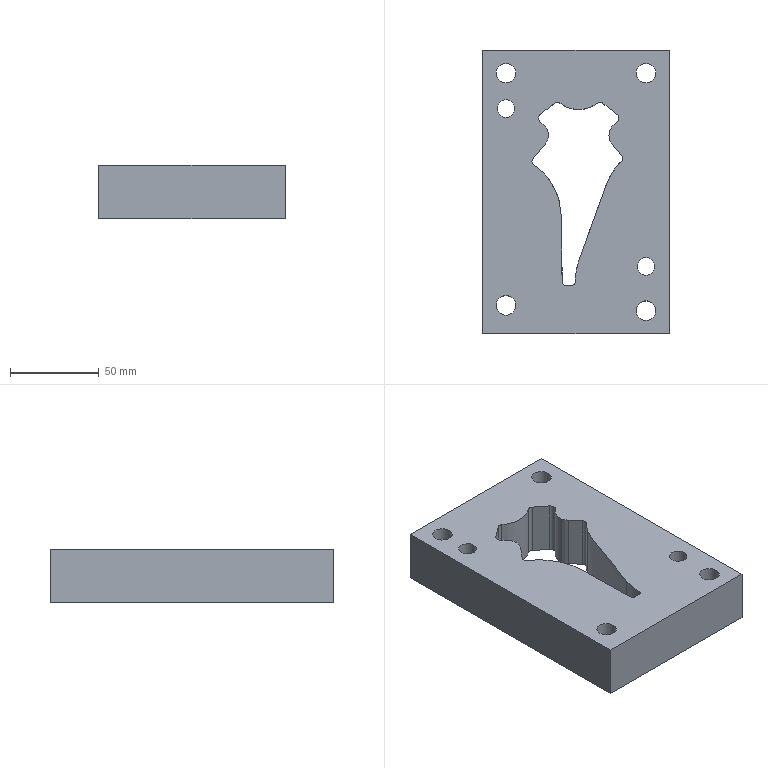Part | STEP file | 204_id722_x_t | 1 solid | 51 faces | box 105 x 160 x 30 mm | volume 399275 mm3 | cylinder 25 | plane 19 | other 7 | commonest cylinder face diameters 5 x8 11 x6 17 x4 6 x2 10 x2 16 x2